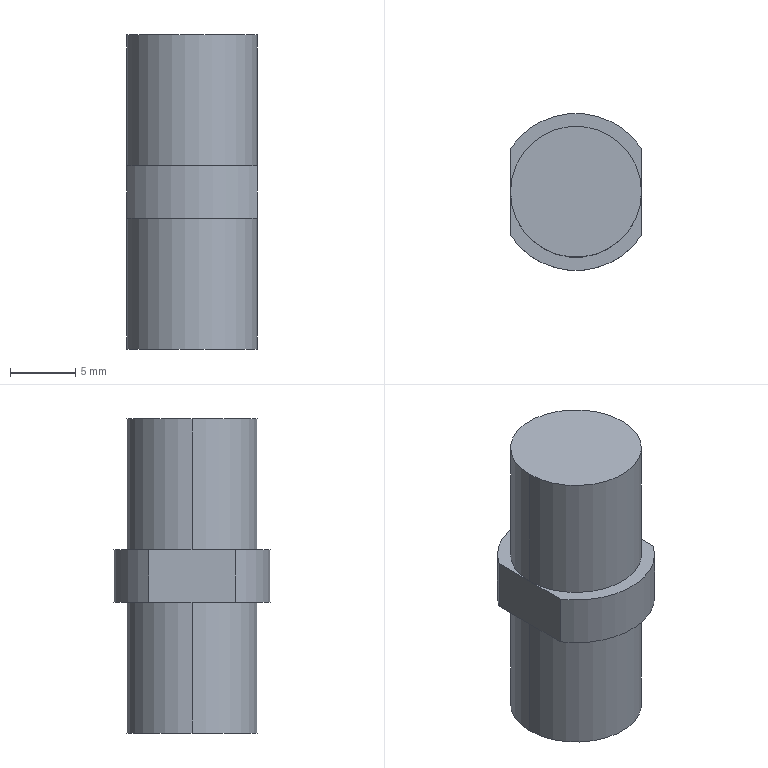Part | SolidWorks | features Revolution 2, Extrusion 1 | 1 solid | 14 faces | box 10 x 12 x 24 mm | volume 1987 mm3 | plane 8 | cylinder 6 | commonest cylinder face diameters 10 x4 12 x2
STEP:
#1=CARTESIAN_POINT('',(-5.,0.,0.));
#2=VERTEX_POINT('',#1);
#3=CARTESIAN_POINT('',(5.,0.,0.));
#4=VERTEX_POINT('',#3);
#5=CARTESIAN_POINT('',(0.,0.,0.));
#6=DIRECTION('',(0.,0.,-1.));
#7=DIRECTION('',(-1.,0.,0.));
#8=AXIS2_PLACEMENT_3D('',#5,#6,#7);
#9=CIRCLE('',#8,5.);
#10=EDGE_CURVE('',#2,#4,#9,.T.);
#11=ORIENTED_EDGE('',*,*,#10,.T.);
#12=CARTESIAN_POINT('',(5.,0.,-10.));
#13=VERTEX_POINT('',#12);
#14=CARTESIAN_POINT('',(5.,0.,0.));
#15=DIRECTION('',(0.,0.,-1.));
#16=VECTOR('',#15,1000.);
#17=LINE('',#14,#16);
#18=EDGE_CURVE('',#4,#13,#17,.T.);
#19=ORIENTED_EDGE('',*,*,#18,.T.);
#20=CARTESIAN_POINT('',(-5.,0.,-10.));
#21=VERTEX_POINT('',#20);
#22=CARTESIAN_POINT('',(0.,0.,-10.));
#23=DIRECTION('',(0.,0.,-1.));
#24=DIRECTION('',(-1.,0.,0.));
#25=AXIS2_PLACEMENT_3D('',#22,#23,#24);
#26=CIRCLE('',#25,5.);
#27=EDGE_CURVE('',#21,#13,#26,.T.);
#28=ORIENTED_EDGE('',*,*,#27,.F.);
#29=CARTESIAN_POINT('',(-5.,0.,0.));
#30=DIRECTION('',(0.,0.,-1.));
#31=VECTOR('',#30,1000.);
#32=LINE('',#29,#31);
#33=EDGE_CURVE('',#2,#21,#32,.T.);
#34=ORIENTED_EDGE('',*,*,#33,.F.);
#35=EDGE_LOOP('',(#11,#19,#28,#34));
#36=FACE_OUTER_BOUND('',#35,.T.);
#37=CARTESIAN_POINT('',(0.,0.,0.));
#38=DIRECTION('',(0.,0.,-1.));
#39=DIRECTION('',(-1.,0.,0.));
#40=AXIS2_PLACEMENT_3D('',#37,#38,#39);
#41=CYLINDRICAL_SURFACE('',#40,5.);
#42=ADVANCED_FACE('',(#36),#41,.T.);
#43=CARTESIAN_POINT('',(5.,0.,4.));
#44=VERTEX_POINT('',#43);
#45=CARTESIAN_POINT('',(-5.,0.,4.));
#46=VERTEX_POINT('',#45);
#47=CARTESIAN_POINT('',(0.,0.,4.));
#48=DIRECTION('',(0.,0.,1.));
#49=DIRECTION('',(1.,0.,0.));
#50=AXIS2_PLACEMENT_3D('',#47,#48,#49);
#51=CIRCLE('',#50,5.);
#52=EDGE_CURVE('',#44,#46,#51,.T.);
#53=ORIENTED_EDGE('',*,*,#52,.T.);
#54=CARTESIAN_POINT('',(-5.,0.,14.));
#55=VERTEX_POINT('',#54);
#56=CARTESIAN_POINT('',(-5.,0.,4.));
#57=DIRECTION('',(0.,0.,1.));
#58=VECTOR('',#57,1000.);
#59=LINE('',#56,#58);
#60=EDGE_CURVE('',#46,#55,#59,.T.);
#61=ORIENTED_EDGE('',*,*,#60,.T.);
#62=CARTESIAN_POINT('',(5.,0.,14.));
#63=VERTEX_POINT('',#62);
#64=CARTESIAN_POINT('',(0.,0.,14.));
#65=DIRECTION('',(0.,0.,1.));
#66=DIRECTION('',(1.,0.,0.));
#67=AXIS2_PLACEMENT_3D('',#64,#65,#66);
#68=CIRCLE('',#67,5.);
#69=EDGE_CURVE('',#63,#55,#68,.T.);
#70=ORIENTED_EDGE('',*,*,#69,.F.);
#71=CARTESIAN_POINT('',(5.,0.,4.));
#72=DIRECTION('',(0.,0.,1.));
#73=VECTOR('',#72,1000.);
#74=LINE('',#71,#73);
#75=EDGE_CURVE('',#44,#63,#74,.T.);
#76=ORIENTED_EDGE('',*,*,#75,.F.);
#77=EDGE_LOOP('',(#53,#61,#70,#76));
#78=FACE_OUTER_BOUND('',#77,.T.);
#79=CARTESIAN_POINT('',(0.,0.,4.));
#80=DIRECTION('',(0.,0.,1.));
#81=DIRECTION('',(1.,0.,0.));
#82=AXIS2_PLACEMENT_3D('',#79,#80,#81);
#83=CYLINDRICAL_SURFACE('',#82,5.);
#84=ADVANCED_FACE('',(#78),#83,.T.);
#85=ORIENTED_EDGE('',*,*,#10,.F.);
#86=CARTESIAN_POINT('',(-5.,3.317,0.));
#87=VERTEX_POINT('',#86);
#88=CARTESIAN_POINT('',(-5.,3.317,0.));
#89=DIRECTION('',(0.,-1.,0.));
#90=VECTOR('',#89,1000.);
#91=LINE('',#88,#90);
#92=EDGE_CURVE('',#87,#2,#91,.T.);
#93=ORIENTED_EDGE('',*,*,#92,.F.);
#94=CARTESIAN_POINT('',(5.,3.317,0.));
#95=VERTEX_POINT('',#94);
#96=CARTESIAN_POINT('',(0.,0.,0.));
#97=DIRECTION('',(0.,0.,1.));
#98=DIRECTION('',(1.,0.,0.));
#99=AXIS2_PLACEMENT_3D('',#96,#97,#98);
#100=CIRCLE('',#99,6.);
#101=EDGE_CURVE('',#95,#87,#100,.T.);
#102=ORIENTED_EDGE('',*,*,#101,.F.);
#103=CARTESIAN_POINT('',(5.,-3.317,0.));
#104=DIRECTION('',(0.,1.,0.));
#105=VECTOR('',#104,1000.);
#106=LINE('',#103,#105);
#107=EDGE_CURVE('',#4,#95,#106,.T.);
#108=ORIENTED_EDGE('',*,*,#107,.F.);
#109=EDGE_LOOP('',(#85,#93,#102,#108));
#110=FACE_OUTER_BOUND('',#109,.T.);
#111=CARTESIAN_POINT('',(0.,0.,0.));
#112=DIRECTION('',(0.,0.,1.));
#113=DIRECTION('',(1.,0.,0.));
#114=AXIS2_PLACEMENT_3D('',#111,#112,#113);
#115=PLANE('',#114);
#116=ADVANCED_FACE('',(#110),#115,.F.);
#117=ORIENTED_EDGE('',*,*,#52,.F.);
#118=CARTESIAN_POINT('',(5.,3.317,4.));
#119=VERTEX_POINT('',#118);
#120=CARTESIAN_POINT('',(5.,-3.317,4.));
#121=DIRECTION('',(0.,1.,0.));
#122=VECTOR('',#121,1000.);
#123=LINE('',#120,#122);
#124=EDGE_CURVE('',#44,#119,#123,.T.);
#125=ORIENTED_EDGE('',*,*,#124,.T.);
#126=CARTESIAN_POINT('',(-5.,3.317,4.));
#127=VERTEX_POINT('',#126);
#128=CARTESIAN_POINT('',(0.,0.,4.));
#129=DIRECTION('',(0.,0.,1.));
#130=DIRECTION('',(1.,0.,0.));
#131=AXIS2_PLACEMENT_3D('',#128,#129,#130);
#132=CIRCLE('',#131,6.);
#133=EDGE_CURVE('',#119,#127,#132,.T.);
#134=ORIENTED_EDGE('',*,*,#133,.T.);
#135=CARTESIAN_POINT('',(-5.,3.317,4.));
#136=DIRECTION('',(0.,-1.,0.));
#137=VECTOR('',#136,1000.);
#138=LINE('',#135,#137);
#139=EDGE_CURVE('',#127,#46,#138,.T.);
#140=ORIENTED_EDGE('',*,*,#139,.T.);
#141=EDGE_LOOP('',(#117,#125,#134,#140));
#142=FACE_OUTER_BOUND('',#141,.T.);
#143=CARTESIAN_POINT('',(0.,0.,4.));
#144=DIRECTION('',(0.,0.,1.));
#145=DIRECTION('',(1.,0.,0.));
#146=AXIS2_PLACEMENT_3D('',#143,#144,#145);
#147=PLANE('',#146);
#148=ADVANCED_FACE('',(#142),#147,.T.);
#149=CARTESIAN_POINT('',(-5.,-3.317,4.));
#150=VERTEX_POINT('',#149);
#151=CARTESIAN_POINT('',(5.,-3.317,4.));
#152=VERTEX_POINT('',#151);
#153=CARTESIAN_POINT('',(0.,0.,4.));
#154=DIRECTION('',(0.,0.,1.));
#155=DIRECTION('',(1.,0.,0.));
#156=AXIS2_PLACEMENT_3D('',#153,#154,#155);
#157=CIRCLE('',#156,6.);
#158=EDGE_CURVE('',#150,#152,#157,.T.);
#159=ORIENTED_EDGE('',*,*,#158,.F.);
#160=CARTESIAN_POINT('',(-5.,-3.317,0.));
#161=VERTEX_POINT('',#160);
#162=CARTESIAN_POINT('',(-5.,-3.317,0.));
#163=DIRECTION('',(0.,0.,1.));
#164=VECTOR('',#163,1000.);
#165=LINE('',#162,#164);
#166=EDGE_CURVE('',#161,#150,#165,.T.);
#167=ORIENTED_EDGE('',*,*,#166,.F.);
#168=CARTESIAN_POINT('',(5.,-3.317,0.));
#169=VERTEX_POINT('',#168);
#170=CARTESIAN_POINT('',(0.,0.,0.));
#171=DIRECTION('',(0.,0.,1.));
#172=DIRECTION('',(1.,0.,0.));
#173=AXIS2_PLACEMENT_3D('',#170,#171,#172);
#174=CIRCLE('',#173,6.);
#175=EDGE_CURVE('',#161,#169,#174,.T.);
#176=ORIENTED_EDGE('',*,*,#175,.T.);
#177=CARTESIAN_POINT('',(5.,-3.317,0.));
#178=DIRECTION('',(0.,0.,1.));
#179=VECTOR('',#178,1000.);
#180=LINE('',#177,#179);
#181=EDGE_CURVE('',#169,#152,#180,.T.);
#182=ORIENTED_EDGE('',*,*,#181,.T.);
#183=EDGE_LOOP('',(#159,#167,#176,#182));
#184=FACE_OUTER_BOUND('',#183,.T.);
#185=CARTESIAN_POINT('',(0.,0.,0.));
#186=DIRECTION('',(0.,0.,1.));
#187=DIRECTION('',(1.,0.,0.));
#188=AXIS2_PLACEMENT_3D('',#185,#186,#187);
#189=CYLINDRICAL_SURFACE('',#188,6.);
#190=ADVANCED_FACE('',(#184),#189,.T.);
#191=ORIENTED_EDGE('',*,*,#139,.F.);
#192=CARTESIAN_POINT('',(-5.,3.317,0.));
#193=DIRECTION('',(0.,0.,1.));
#194=VECTOR('',#193,1000.);
#195=LINE('',#192,#194);
#196=EDGE_CURVE('',#87,#127,#195,.T.);
#197=ORIENTED_EDGE('',*,*,#196,.F.);
#198=ORIENTED_EDGE('',*,*,#92,.T.);
#199=CARTESIAN_POINT('',(-5.,3.317,0.));
#200=DIRECTION('',(0.,-1.,0.));
#201=VECTOR('',#200,1000.);
#202=LINE('',#199,#201);
#203=EDGE_CURVE('',#2,#161,#202,.T.);
#204=ORIENTED_EDGE('',*,*,#203,.T.);
#205=ORIENTED_EDGE('',*,*,#166,.T.);
#206=CARTESIAN_POINT('',(-5.,3.317,4.));
#207=DIRECTION('',(0.,-1.,0.));
#208=VECTOR('',#207,1000.);
#209=LINE('',#206,#208);
#210=EDGE_CURVE('',#46,#150,#209,.T.);
#211=ORIENTED_EDGE('',*,*,#210,.F.);
#212=EDGE_LOOP('',(#191,#197,#198,#204,#205,#211));
#213=FACE_OUTER_BOUND('',#212,.T.);
#214=CARTESIAN_POINT('',(-5.,3.317,0.));
#215=DIRECTION('',(-1.,0.,0.));
#216=DIRECTION('',(0.,0.,1.));
#217=AXIS2_PLACEMENT_3D('',#214,#215,#216);
#218=PLANE('',#217);
#219=ADVANCED_FACE('',(#213),#218,.T.);
#220=ORIENTED_EDGE('',*,*,#133,.F.);
#221=CARTESIAN_POINT('',(5.,3.317,0.));
#222=DIRECTION('',(0.,0.,1.));
#223=VECTOR('',#222,1000.);
#224=LINE('',#221,#223);
#225=EDGE_CURVE('',#95,#119,#224,.T.);
#226=ORIENTED_EDGE('',*,*,#225,.F.);
#227=ORIENTED_EDGE('',*,*,#101,.T.);
#228=ORIENTED_EDGE('',*,*,#196,.T.);
#229=EDGE_LOOP('',(#220,#226,#227,#228));
#230=FACE_OUTER_BOUND('',#229,.T.);
#231=CARTESIAN_POINT('',(0.,0.,0.));
#232=DIRECTION('',(0.,0.,1.));
#233=DIRECTION('',(1.,0.,0.));
#234=AXIS2_PLACEMENT_3D('',#231,#232,#233);
#235=CYLINDRICAL_SURFACE('',#234,6.);
#236=ADVANCED_FACE('',(#230),#235,.T.);
#237=CARTESIAN_POINT('',(5.,-3.317,4.));
#238=DIRECTION('',(0.,1.,0.));
#239=VECTOR('',#238,1000.);
#240=LINE('',#237,#239);
#241=EDGE_CURVE('',#152,#44,#240,.T.);
#242=ORIENTED_EDGE('',*,*,#241,.F.);
#243=ORIENTED_EDGE('',*,*,#181,.F.);
#244=CARTESIAN_POINT('',(5.,-3.317,0.));
#245=DIRECTION('',(0.,1.,0.));
#246=VECTOR('',#245,1000.);
#247=LINE('',#244,#246);
#248=EDGE_CURVE('',#169,#4,#247,.T.);
#249=ORIENTED_EDGE('',*,*,#248,.T.);
#250=ORIENTED_EDGE('',*,*,#107,.T.);
#251=ORIENTED_EDGE('',*,*,#225,.T.);
#252=ORIENTED_EDGE('',*,*,#124,.F.);
#253=EDGE_LOOP('',(#242,#243,#249,#250,#251,#252));
#254=FACE_OUTER_BOUND('',#253,.T.);
#255=CARTESIAN_POINT('',(5.,-3.317,0.));
#256=DIRECTION('',(1.,0.,0.));
#257=DIRECTION('',(0.,0.,-1.));
#258=AXIS2_PLACEMENT_3D('',#255,#256,#257);
#259=PLANE('',#258);
#260=ADVANCED_FACE('',(#254),#259,.T.);
#261=CARTESIAN_POINT('',(0.,0.,0.));
#262=DIRECTION('',(0.,0.,-1.));
#263=DIRECTION('',(-1.,0.,0.));
#264=AXIS2_PLACEMENT_3D('',#261,#262,#263);
#265=CIRCLE('',#264,5.);
#266=EDGE_CURVE('',#4,#2,#265,.T.);
#267=ORIENTED_EDGE('',*,*,#266,.F.);
#268=ORIENTED_EDGE('',*,*,#248,.F.);
#269=ORIENTED_EDGE('',*,*,#175,.F.);
#270=ORIENTED_EDGE('',*,*,#203,.F.);
#271=EDGE_LOOP('',(#267,#268,#269,#270));
#272=FACE_OUTER_BOUND('',#271,.T.);
#273=CARTESIAN_POINT('',(0.,0.,0.));
#274=DIRECTION('',(0.,0.,1.));
#275=DIRECTION('',(1.,0.,0.));
#276=AXIS2_PLACEMENT_3D('',#273,#274,#275);
#277=PLANE('',#276);
#278=ADVANCED_FACE('',(#272),#277,.F.);
#279=CARTESIAN_POINT('',(0.,0.,4.));
#280=DIRECTION('',(0.,0.,1.));
#281=DIRECTION('',(1.,0.,0.));
#282=AXIS2_PLACEMENT_3D('',#279,#280,#281);
#283=CIRCLE('',#282,5.);
#284=EDGE_CURVE('',#46,#44,#283,.T.);
#285=ORIENTED_EDGE('',*,*,#284,.F.);
#286=ORIENTED_EDGE('',*,*,#210,.T.);
#287=ORIENTED_EDGE('',*,*,#158,.T.);
#288=ORIENTED_EDGE('',*,*,#241,.T.);
#289=EDGE_LOOP('',(#285,#286,#287,#288));
#290=FACE_OUTER_BOUND('',#289,.T.);
#291=CARTESIAN_POINT('',(0.,0.,4.));
#292=DIRECTION('',(0.,0.,1.));
#293=DIRECTION('',(1.,0.,0.));
#294=AXIS2_PLACEMENT_3D('',#291,#292,#293);
#295=PLANE('',#294);
#296=ADVANCED_FACE('',(#290),#295,.T.);
#297=ORIENTED_EDGE('',*,*,#60,.F.);
#298=ORIENTED_EDGE('',*,*,#284,.T.);
#299=ORIENTED_EDGE('',*,*,#75,.T.);
#300=CARTESIAN_POINT('',(0.,0.,14.));
#301=DIRECTION('',(0.,0.,1.));
#302=DIRECTION('',(1.,0.,0.));
#303=AXIS2_PLACEMENT_3D('',#300,#301,#302);
#304=CIRCLE('',#303,5.);
#305=EDGE_CURVE('',#55,#63,#304,.T.);
#306=ORIENTED_EDGE('',*,*,#305,.F.);
#307=EDGE_LOOP('',(#297,#298,#299,#306));
#308=FACE_OUTER_BOUND('',#307,.T.);
#309=CARTESIAN_POINT('',(0.,0.,4.));
#310=DIRECTION('',(0.,0.,1.));
#311=DIRECTION('',(1.,0.,0.));
#312=AXIS2_PLACEMENT_3D('',#309,#310,#311);
#313=CYLINDRICAL_SURFACE('',#312,5.);
#314=ADVANCED_FACE('',(#308),#313,.T.);
#315=ORIENTED_EDGE('',*,*,#69,.T.);
#316=ORIENTED_EDGE('',*,*,#305,.T.);
#317=EDGE_LOOP('',(#315,#316));
#318=FACE_OUTER_BOUND('',#317,.T.);
#319=CARTESIAN_POINT('',(0.,0.,14.));
#320=DIRECTION('',(0.,0.,1.));
#321=DIRECTION('',(1.,0.,0.));
#322=AXIS2_PLACEMENT_3D('',#319,#320,#321);
#323=PLANE('',#322);
#324=ADVANCED_FACE('',(#318),#323,.T.);
#325=ORIENTED_EDGE('',*,*,#18,.F.);
#326=ORIENTED_EDGE('',*,*,#266,.T.);
#327=ORIENTED_EDGE('',*,*,#33,.T.);
#328=CARTESIAN_POINT('',(0.,0.,-10.));
#329=DIRECTION('',(0.,0.,-1.));
#330=DIRECTION('',(-1.,0.,0.));
#331=AXIS2_PLACEMENT_3D('',#328,#329,#330);
#332=CIRCLE('',#331,5.);
#333=EDGE_CURVE('',#13,#21,#332,.T.);
#334=ORIENTED_EDGE('',*,*,#333,.F.);
#335=EDGE_LOOP('',(#325,#326,#327,#334));
#336=FACE_OUTER_BOUND('',#335,.T.);
#337=CARTESIAN_POINT('',(0.,0.,0.));
#338=DIRECTION('',(0.,0.,-1.));
#339=DIRECTION('',(-1.,0.,0.));
#340=AXIS2_PLACEMENT_3D('',#337,#338,#339);
#341=CYLINDRICAL_SURFACE('',#340,5.);
#342=ADVANCED_FACE('',(#336),#341,.T.);
#343=ORIENTED_EDGE('',*,*,#27,.T.);
#344=ORIENTED_EDGE('',*,*,#333,.T.);
#345=EDGE_LOOP('',(#343,#344));
#346=FACE_OUTER_BOUND('',#345,.T.);
#347=CARTESIAN_POINT('',(0.,0.,-10.));
#348=DIRECTION('',(0.,0.,-1.));
#349=DIRECTION('',(-1.,0.,0.));
#350=AXIS2_PLACEMENT_3D('',#347,#348,#349);
#351=PLANE('',#350);
#352=ADVANCED_FACE('',(#346),#351,.T.);
#353=CLOSED_SHELL('',(#42,#84,#116,#148,#190,#219,#236,#260,#278,#296,#314,#324,#342,#352));
#354=MANIFOLD_SOLID_BREP('',#353);
#355=CARTESIAN_POINT('',(0.,0.,0.));
#356=DIRECTION('',(0.,0.,1.));
#357=DIRECTION('',(1.,0.,0.));
#358=AXIS2_PLACEMENT_3D('',#355,#356,#357);
#359=(LENGTH_UNIT()NAMED_UNIT(*)SI_UNIT(.MILLI.,.METRE.));
#360=UNCERTAINTY_MEASURE_WITH_UNIT(LENGTH_MEASURE(0.00001),#359,'','');
#361=(NAMED_UNIT(*)PLANE_ANGLE_UNIT()SI_UNIT($,.RADIAN.));
#362=(NAMED_UNIT(*)SI_UNIT($,.STERADIAN.)SOLID_ANGLE_UNIT());
#363=(GEOMETRIC_REPRESENTATION_CONTEXT(3)GLOBAL_UNCERTAINTY_ASSIGNED_CONTEXT((#360))GLOBAL_UNIT_ASSIGNED_CONTEXT((#359,#361,#362))REPRESENTATION_CONTEXT('',''));
#364=ADVANCED_BREP_SHAPE_REPRESENTATION('',(#354,#358),#363);